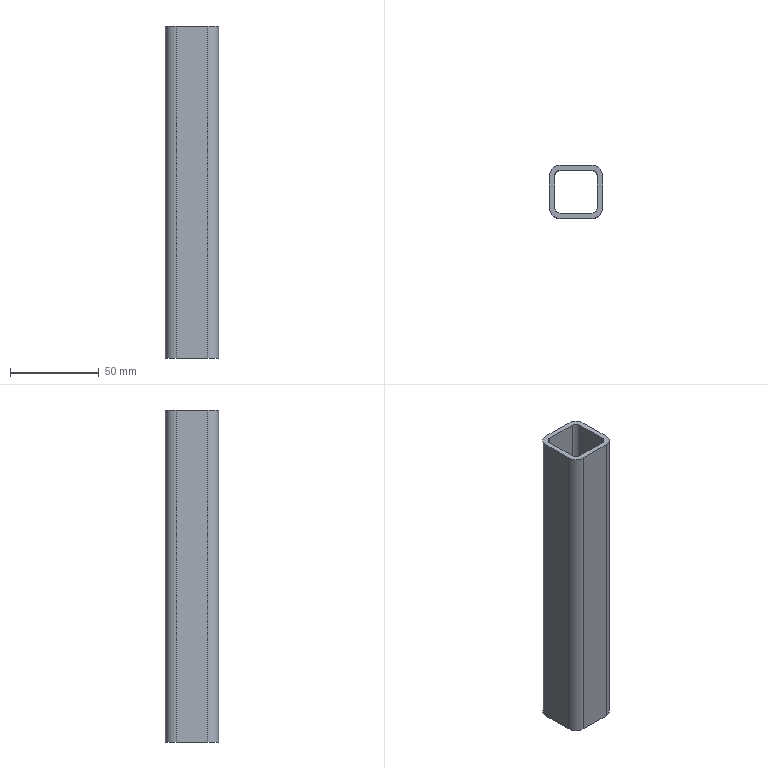Part | SolidWorks | features Attribute 1, Extrusion 1 | 1 solid | 18 faces | box 30 x 30 x 187 mm | volume 56254 mm3 | plane 10 | cylinder 8 | commonest cylinder face diameters 6 x4 12 x4
STEP:
#1=CARTESIAN_POINT('',(-15.,-9.,187.));
#2=VERTEX_POINT('',#1);
#3=CARTESIAN_POINT('',(-9.,-15.,187.));
#4=VERTEX_POINT('',#3);
#5=CARTESIAN_POINT('',(-9.,-9.,187.));
#6=DIRECTION('',(0.,0.,1.));
#7=DIRECTION('',(1.,0.,0.));
#8=AXIS2_PLACEMENT_3D('',#5,#6,#7);
#9=CIRCLE('',#8,6.);
#10=EDGE_CURVE('',#2,#4,#9,.T.);
#11=ORIENTED_EDGE('',*,*,#10,.T.);
#12=CARTESIAN_POINT('',(9.,-15.,187.));
#13=VERTEX_POINT('',#12);
#14=CARTESIAN_POINT('',(-9.,-15.,187.));
#15=DIRECTION('',(1.,0.,0.));
#16=VECTOR('',#15,1000.);
#17=LINE('',#14,#16);
#18=EDGE_CURVE('',#4,#13,#17,.T.);
#19=ORIENTED_EDGE('',*,*,#18,.T.);
#20=CARTESIAN_POINT('',(15.,-9.,187.));
#21=VERTEX_POINT('',#20);
#22=CARTESIAN_POINT('',(9.,-9.,187.));
#23=DIRECTION('',(0.,0.,1.));
#24=DIRECTION('',(1.,0.,0.));
#25=AXIS2_PLACEMENT_3D('',#22,#23,#24);
#26=CIRCLE('',#25,6.);
#27=EDGE_CURVE('',#13,#21,#26,.T.);
#28=ORIENTED_EDGE('',*,*,#27,.T.);
#29=CARTESIAN_POINT('',(15.,9.,187.));
#30=VERTEX_POINT('',#29);
#31=CARTESIAN_POINT('',(15.,9.,187.));
#32=DIRECTION('',(0.,-1.,0.));
#33=VECTOR('',#32,1000.);
#34=LINE('',#31,#33);
#35=EDGE_CURVE('',#30,#21,#34,.T.);
#36=ORIENTED_EDGE('',*,*,#35,.F.);
#37=CARTESIAN_POINT('',(9.,15.,187.));
#38=VERTEX_POINT('',#37);
#39=CARTESIAN_POINT('',(9.,9.,187.));
#40=DIRECTION('',(0.,0.,1.));
#41=DIRECTION('',(1.,0.,0.));
#42=AXIS2_PLACEMENT_3D('',#39,#40,#41);
#43=CIRCLE('',#42,6.);
#44=EDGE_CURVE('',#30,#38,#43,.T.);
#45=ORIENTED_EDGE('',*,*,#44,.T.);
#46=CARTESIAN_POINT('',(-9.,15.,187.));
#47=VERTEX_POINT('',#46);
#48=CARTESIAN_POINT('',(9.,15.,187.));
#49=DIRECTION('',(-1.,0.,0.));
#50=VECTOR('',#49,1000.);
#51=LINE('',#48,#50);
#52=EDGE_CURVE('',#38,#47,#51,.T.);
#53=ORIENTED_EDGE('',*,*,#52,.T.);
#54=CARTESIAN_POINT('',(-15.,9.,187.));
#55=VERTEX_POINT('',#54);
#56=CARTESIAN_POINT('',(-9.,9.,187.));
#57=DIRECTION('',(0.,0.,1.));
#58=DIRECTION('',(1.,0.,0.));
#59=AXIS2_PLACEMENT_3D('',#56,#57,#58);
#60=CIRCLE('',#59,6.);
#61=EDGE_CURVE('',#47,#55,#60,.T.);
#62=ORIENTED_EDGE('',*,*,#61,.T.);
#63=CARTESIAN_POINT('',(-15.,-9.,187.));
#64=DIRECTION('',(0.,1.,0.));
#65=VECTOR('',#64,1000.);
#66=LINE('',#63,#65);
#67=EDGE_CURVE('',#2,#55,#66,.T.);
#68=ORIENTED_EDGE('',*,*,#67,.F.);
#69=EDGE_LOOP('',(#11,#19,#28,#36,#45,#53,#62,#68));
#70=FACE_OUTER_BOUND('',#69,.T.);
#71=CARTESIAN_POINT('',(-9.,-12.,187.));
#72=VERTEX_POINT('',#71);
#73=CARTESIAN_POINT('',(9.,-12.,187.));
#74=VERTEX_POINT('',#73);
#75=CARTESIAN_POINT('',(-9.,-12.,187.));
#76=DIRECTION('',(1.,0.,0.));
#77=VECTOR('',#76,1000.);
#78=LINE('',#75,#77);
#79=EDGE_CURVE('',#72,#74,#78,.T.);
#80=ORIENTED_EDGE('',*,*,#79,.F.);
#81=CARTESIAN_POINT('',(-12.,-9.,187.));
#82=VERTEX_POINT('',#81);
#83=CARTESIAN_POINT('',(-9.,-9.,187.));
#84=DIRECTION('',(0.,0.,1.));
#85=DIRECTION('',(1.,0.,0.));
#86=AXIS2_PLACEMENT_3D('',#83,#84,#85);
#87=CIRCLE('',#86,3.);
#88=EDGE_CURVE('',#82,#72,#87,.T.);
#89=ORIENTED_EDGE('',*,*,#88,.F.);
#90=CARTESIAN_POINT('',(-12.,9.,187.));
#91=VERTEX_POINT('',#90);
#92=CARTESIAN_POINT('',(-12.,-9.,187.));
#93=DIRECTION('',(0.,1.,0.));
#94=VECTOR('',#93,1000.);
#95=LINE('',#92,#94);
#96=EDGE_CURVE('',#82,#91,#95,.T.);
#97=ORIENTED_EDGE('',*,*,#96,.T.);
#98=CARTESIAN_POINT('',(-9.,12.,187.));
#99=VERTEX_POINT('',#98);
#100=CARTESIAN_POINT('',(-9.,9.,187.));
#101=DIRECTION('',(0.,0.,1.));
#102=DIRECTION('',(1.,0.,0.));
#103=AXIS2_PLACEMENT_3D('',#100,#101,#102);
#104=CIRCLE('',#103,3.);
#105=EDGE_CURVE('',#99,#91,#104,.T.);
#106=ORIENTED_EDGE('',*,*,#105,.F.);
#107=CARTESIAN_POINT('',(9.,12.,187.));
#108=VERTEX_POINT('',#107);
#109=CARTESIAN_POINT('',(9.,12.,187.));
#110=DIRECTION('',(-1.,0.,0.));
#111=VECTOR('',#110,1000.);
#112=LINE('',#109,#111);
#113=EDGE_CURVE('',#108,#99,#112,.T.);
#114=ORIENTED_EDGE('',*,*,#113,.F.);
#115=CARTESIAN_POINT('',(12.,9.,187.));
#116=VERTEX_POINT('',#115);
#117=CARTESIAN_POINT('',(9.,9.,187.));
#118=DIRECTION('',(0.,0.,1.));
#119=DIRECTION('',(1.,0.,0.));
#120=AXIS2_PLACEMENT_3D('',#117,#118,#119);
#121=CIRCLE('',#120,3.);
#122=EDGE_CURVE('',#116,#108,#121,.T.);
#123=ORIENTED_EDGE('',*,*,#122,.F.);
#124=CARTESIAN_POINT('',(12.,-9.,187.));
#125=VERTEX_POINT('',#124);
#126=CARTESIAN_POINT('',(12.,9.,187.));
#127=DIRECTION('',(0.,-1.,0.));
#128=VECTOR('',#127,1000.);
#129=LINE('',#126,#128);
#130=EDGE_CURVE('',#116,#125,#129,.T.);
#131=ORIENTED_EDGE('',*,*,#130,.T.);
#132=CARTESIAN_POINT('',(9.,-9.,187.));
#133=DIRECTION('',(0.,0.,1.));
#134=DIRECTION('',(1.,0.,0.));
#135=AXIS2_PLACEMENT_3D('',#132,#133,#134);
#136=CIRCLE('',#135,3.);
#137=EDGE_CURVE('',#74,#125,#136,.T.);
#138=ORIENTED_EDGE('',*,*,#137,.F.);
#139=EDGE_LOOP('',(#80,#89,#97,#106,#114,#123,#131,#138));
#140=FACE_BOUND('',#139,.T.);
#141=CARTESIAN_POINT('',(-9.,-9.,187.));
#142=DIRECTION('',(0.,0.,1.));
#143=DIRECTION('',(1.,0.,0.));
#144=AXIS2_PLACEMENT_3D('',#141,#142,#143);
#145=PLANE('',#144);
#146=ADVANCED_FACE('',(#70,#140),#145,.T.);
#147=CARTESIAN_POINT('',(-15.,-9.,0.));
#148=VERTEX_POINT('',#147);
#149=CARTESIAN_POINT('',(-9.,-15.,0.));
#150=VERTEX_POINT('',#149);
#151=CARTESIAN_POINT('',(-9.,-9.,0.));
#152=DIRECTION('',(0.,0.,1.));
#153=DIRECTION('',(1.,0.,0.));
#154=AXIS2_PLACEMENT_3D('',#151,#152,#153);
#155=CIRCLE('',#154,6.);
#156=EDGE_CURVE('',#148,#150,#155,.T.);
#157=ORIENTED_EDGE('',*,*,#156,.F.);
#158=CARTESIAN_POINT('',(-15.,9.,0.));
#159=VERTEX_POINT('',#158);
#160=CARTESIAN_POINT('',(-15.,-9.,0.));
#161=DIRECTION('',(0.,1.,0.));
#162=VECTOR('',#161,1000.);
#163=LINE('',#160,#162);
#164=EDGE_CURVE('',#148,#159,#163,.T.);
#165=ORIENTED_EDGE('',*,*,#164,.T.);
#166=CARTESIAN_POINT('',(-9.,15.,0.));
#167=VERTEX_POINT('',#166);
#168=CARTESIAN_POINT('',(-9.,9.,0.));
#169=DIRECTION('',(0.,0.,1.));
#170=DIRECTION('',(1.,0.,0.));
#171=AXIS2_PLACEMENT_3D('',#168,#169,#170);
#172=CIRCLE('',#171,6.);
#173=EDGE_CURVE('',#167,#159,#172,.T.);
#174=ORIENTED_EDGE('',*,*,#173,.F.);
#175=CARTESIAN_POINT('',(9.,15.,0.));
#176=VERTEX_POINT('',#175);
#177=CARTESIAN_POINT('',(9.,15.,0.));
#178=DIRECTION('',(-1.,0.,0.));
#179=VECTOR('',#178,1000.);
#180=LINE('',#177,#179);
#181=EDGE_CURVE('',#176,#167,#180,.T.);
#182=ORIENTED_EDGE('',*,*,#181,.F.);
#183=CARTESIAN_POINT('',(15.,9.,0.));
#184=VERTEX_POINT('',#183);
#185=CARTESIAN_POINT('',(9.,9.,0.));
#186=DIRECTION('',(0.,0.,1.));
#187=DIRECTION('',(1.,0.,0.));
#188=AXIS2_PLACEMENT_3D('',#185,#186,#187);
#189=CIRCLE('',#188,6.);
#190=EDGE_CURVE('',#184,#176,#189,.T.);
#191=ORIENTED_EDGE('',*,*,#190,.F.);
#192=CARTESIAN_POINT('',(15.,-9.,0.));
#193=VERTEX_POINT('',#192);
#194=CARTESIAN_POINT('',(15.,9.,0.));
#195=DIRECTION('',(0.,-1.,0.));
#196=VECTOR('',#195,1000.);
#197=LINE('',#194,#196);
#198=EDGE_CURVE('',#184,#193,#197,.T.);
#199=ORIENTED_EDGE('',*,*,#198,.T.);
#200=CARTESIAN_POINT('',(9.,-15.,0.));
#201=VERTEX_POINT('',#200);
#202=CARTESIAN_POINT('',(9.,-9.,0.));
#203=DIRECTION('',(0.,0.,1.));
#204=DIRECTION('',(1.,0.,0.));
#205=AXIS2_PLACEMENT_3D('',#202,#203,#204);
#206=CIRCLE('',#205,6.);
#207=EDGE_CURVE('',#201,#193,#206,.T.);
#208=ORIENTED_EDGE('',*,*,#207,.F.);
#209=CARTESIAN_POINT('',(-9.,-15.,0.));
#210=DIRECTION('',(1.,0.,0.));
#211=VECTOR('',#210,1000.);
#212=LINE('',#209,#211);
#213=EDGE_CURVE('',#150,#201,#212,.T.);
#214=ORIENTED_EDGE('',*,*,#213,.F.);
#215=EDGE_LOOP('',(#157,#165,#174,#182,#191,#199,#208,#214));
#216=FACE_OUTER_BOUND('',#215,.T.);
#217=CARTESIAN_POINT('',(-12.,-9.,0.));
#218=VERTEX_POINT('',#217);
#219=CARTESIAN_POINT('',(-9.,-12.,0.));
#220=VERTEX_POINT('',#219);
#221=CARTESIAN_POINT('',(-9.,-9.,0.));
#222=DIRECTION('',(0.,0.,1.));
#223=DIRECTION('',(1.,0.,0.));
#224=AXIS2_PLACEMENT_3D('',#221,#222,#223);
#225=CIRCLE('',#224,3.);
#226=EDGE_CURVE('',#218,#220,#225,.T.);
#227=ORIENTED_EDGE('',*,*,#226,.T.);
#228=CARTESIAN_POINT('',(9.,-12.,0.));
#229=VERTEX_POINT('',#228);
#230=CARTESIAN_POINT('',(-9.,-12.,0.));
#231=DIRECTION('',(1.,0.,0.));
#232=VECTOR('',#231,1000.);
#233=LINE('',#230,#232);
#234=EDGE_CURVE('',#220,#229,#233,.T.);
#235=ORIENTED_EDGE('',*,*,#234,.T.);
#236=CARTESIAN_POINT('',(12.,-9.,0.));
#237=VERTEX_POINT('',#236);
#238=CARTESIAN_POINT('',(9.,-9.,0.));
#239=DIRECTION('',(0.,0.,1.));
#240=DIRECTION('',(1.,0.,0.));
#241=AXIS2_PLACEMENT_3D('',#238,#239,#240);
#242=CIRCLE('',#241,3.);
#243=EDGE_CURVE('',#229,#237,#242,.T.);
#244=ORIENTED_EDGE('',*,*,#243,.T.);
#245=CARTESIAN_POINT('',(12.,9.,0.));
#246=VERTEX_POINT('',#245);
#247=CARTESIAN_POINT('',(12.,9.,0.));
#248=DIRECTION('',(0.,-1.,0.));
#249=VECTOR('',#248,1000.);
#250=LINE('',#247,#249);
#251=EDGE_CURVE('',#246,#237,#250,.T.);
#252=ORIENTED_EDGE('',*,*,#251,.F.);
#253=CARTESIAN_POINT('',(9.,12.,0.));
#254=VERTEX_POINT('',#253);
#255=CARTESIAN_POINT('',(9.,9.,0.));
#256=DIRECTION('',(0.,0.,1.));
#257=DIRECTION('',(1.,0.,0.));
#258=AXIS2_PLACEMENT_3D('',#255,#256,#257);
#259=CIRCLE('',#258,3.);
#260=EDGE_CURVE('',#246,#254,#259,.T.);
#261=ORIENTED_EDGE('',*,*,#260,.T.);
#262=CARTESIAN_POINT('',(-9.,12.,0.));
#263=VERTEX_POINT('',#262);
#264=CARTESIAN_POINT('',(9.,12.,0.));
#265=DIRECTION('',(-1.,0.,0.));
#266=VECTOR('',#265,1000.);
#267=LINE('',#264,#266);
#268=EDGE_CURVE('',#254,#263,#267,.T.);
#269=ORIENTED_EDGE('',*,*,#268,.T.);
#270=CARTESIAN_POINT('',(-12.,9.,0.));
#271=VERTEX_POINT('',#270);
#272=CARTESIAN_POINT('',(-9.,9.,0.));
#273=DIRECTION('',(0.,0.,1.));
#274=DIRECTION('',(1.,0.,0.));
#275=AXIS2_PLACEMENT_3D('',#272,#273,#274);
#276=CIRCLE('',#275,3.);
#277=EDGE_CURVE('',#263,#271,#276,.T.);
#278=ORIENTED_EDGE('',*,*,#277,.T.);
#279=CARTESIAN_POINT('',(-12.,-9.,0.));
#280=DIRECTION('',(0.,1.,0.));
#281=VECTOR('',#280,1000.);
#282=LINE('',#279,#281);
#283=EDGE_CURVE('',#218,#271,#282,.T.);
#284=ORIENTED_EDGE('',*,*,#283,.F.);
#285=EDGE_LOOP('',(#227,#235,#244,#252,#261,#269,#278,#284));
#286=FACE_BOUND('',#285,.T.);
#287=CARTESIAN_POINT('',(-9.,-9.,0.));
#288=DIRECTION('',(0.,0.,1.));
#289=DIRECTION('',(1.,0.,0.));
#290=AXIS2_PLACEMENT_3D('',#287,#288,#289);
#291=PLANE('',#290);
#292=ADVANCED_FACE('',(#216,#286),#291,.F.);
#293=ORIENTED_EDGE('',*,*,#156,.T.);
#294=CARTESIAN_POINT('',(-9.,-15.,187.));
#295=DIRECTION('',(0.,0.,-1.));
#296=VECTOR('',#295,1000.);
#297=LINE('',#294,#296);
#298=EDGE_CURVE('',#4,#150,#297,.T.);
#299=ORIENTED_EDGE('',*,*,#298,.F.);
#300=ORIENTED_EDGE('',*,*,#10,.F.);
#301=CARTESIAN_POINT('',(-15.,-9.,187.));
#302=DIRECTION('',(0.,0.,-1.));
#303=VECTOR('',#302,1000.);
#304=LINE('',#301,#303);
#305=EDGE_CURVE('',#2,#148,#304,.T.);
#306=ORIENTED_EDGE('',*,*,#305,.T.);
#307=EDGE_LOOP('',(#293,#299,#300,#306));
#308=FACE_OUTER_BOUND('',#307,.T.);
#309=CARTESIAN_POINT('',(-9.,-9.,187.));
#310=DIRECTION('',(0.,0.,-1.));
#311=DIRECTION('',(-1.,0.,0.));
#312=AXIS2_PLACEMENT_3D('',#309,#310,#311);
#313=CYLINDRICAL_SURFACE('',#312,6.);
#314=ADVANCED_FACE('',(#308),#313,.T.);
#315=ORIENTED_EDGE('',*,*,#213,.T.);
#316=CARTESIAN_POINT('',(9.,-15.,187.));
#317=DIRECTION('',(0.,0.,-1.));
#318=VECTOR('',#317,1000.);
#319=LINE('',#316,#318);
#320=EDGE_CURVE('',#13,#201,#319,.T.);
#321=ORIENTED_EDGE('',*,*,#320,.F.);
#322=ORIENTED_EDGE('',*,*,#18,.F.);
#323=ORIENTED_EDGE('',*,*,#298,.T.);
#324=EDGE_LOOP('',(#315,#321,#322,#323));
#325=FACE_OUTER_BOUND('',#324,.T.);
#326=CARTESIAN_POINT('',(-9.,-15.,187.));
#327=DIRECTION('',(0.,1.,0.));
#328=DIRECTION('',(0.,0.,1.));
#329=AXIS2_PLACEMENT_3D('',#326,#327,#328);
#330=PLANE('',#329);
#331=ADVANCED_FACE('',(#325),#330,.F.);
#332=ORIENTED_EDGE('',*,*,#207,.T.);
#333=CARTESIAN_POINT('',(15.,-9.,187.));
#334=DIRECTION('',(0.,0.,-1.));
#335=VECTOR('',#334,1000.);
#336=LINE('',#333,#335);
#337=EDGE_CURVE('',#21,#193,#336,.T.);
#338=ORIENTED_EDGE('',*,*,#337,.F.);
#339=ORIENTED_EDGE('',*,*,#27,.F.);
#340=ORIENTED_EDGE('',*,*,#320,.T.);
#341=EDGE_LOOP('',(#332,#338,#339,#340));
#342=FACE_OUTER_BOUND('',#341,.T.);
#343=CARTESIAN_POINT('',(9.,-9.,187.));
#344=DIRECTION('',(0.,0.,-1.));
#345=DIRECTION('',(-1.,0.,0.));
#346=AXIS2_PLACEMENT_3D('',#343,#344,#345);
#347=CYLINDRICAL_SURFACE('',#346,6.);
#348=ADVANCED_FACE('',(#342),#347,.T.);
#349=ORIENTED_EDGE('',*,*,#198,.F.);
#350=CARTESIAN_POINT('',(15.,9.,187.));
#351=DIRECTION('',(0.,0.,-1.));
#352=VECTOR('',#351,1000.);
#353=LINE('',#350,#352);
#354=EDGE_CURVE('',#30,#184,#353,.T.);
#355=ORIENTED_EDGE('',*,*,#354,.F.);
#356=ORIENTED_EDGE('',*,*,#35,.T.);
#357=ORIENTED_EDGE('',*,*,#337,.T.);
#358=EDGE_LOOP('',(#349,#355,#356,#357));
#359=FACE_OUTER_BOUND('',#358,.T.);
#360=CARTESIAN_POINT('',(15.,9.,187.));
#361=DIRECTION('',(1.,0.,0.));
#362=DIRECTION('',(0.,0.,-1.));
#363=AXIS2_PLACEMENT_3D('',#360,#361,#362);
#364=PLANE('',#363);
#365=ADVANCED_FACE('',(#359),#364,.T.);
#366=ORIENTED_EDGE('',*,*,#190,.T.);
#367=CARTESIAN_POINT('',(9.,15.,187.));
#368=DIRECTION('',(0.,0.,-1.));
#369=VECTOR('',#368,1000.);
#370=LINE('',#367,#369);
#371=EDGE_CURVE('',#38,#176,#370,.T.);
#372=ORIENTED_EDGE('',*,*,#371,.F.);
#373=ORIENTED_EDGE('',*,*,#44,.F.);
#374=ORIENTED_EDGE('',*,*,#354,.T.);
#375=EDGE_LOOP('',(#366,#372,#373,#374));
#376=FACE_OUTER_BOUND('',#375,.T.);
#377=CARTESIAN_POINT('',(9.,9.,187.));
#378=DIRECTION('',(0.,0.,-1.));
#379=DIRECTION('',(-1.,0.,0.));
#380=AXIS2_PLACEMENT_3D('',#377,#378,#379);
#381=CYLINDRICAL_SURFACE('',#380,6.);
#382=ADVANCED_FACE('',(#376),#381,.T.);
#383=ORIENTED_EDGE('',*,*,#181,.T.);
#384=CARTESIAN_POINT('',(-9.,15.,187.));
#385=DIRECTION('',(0.,0.,-1.));
#386=VECTOR('',#385,1000.);
#387=LINE('',#384,#386);
#388=EDGE_CURVE('',#47,#167,#387,.T.);
#389=ORIENTED_EDGE('',*,*,#388,.F.);
#390=ORIENTED_EDGE('',*,*,#52,.F.);
#391=ORIENTED_EDGE('',*,*,#371,.T.);
#392=EDGE_LOOP('',(#383,#389,#390,#391));
#393=FACE_OUTER_BOUND('',#392,.T.);
#394=CARTESIAN_POINT('',(9.,15.,187.));
#395=DIRECTION('',(0.,-1.,0.));
#396=DIRECTION('',(0.,0.,-1.));
#397=AXIS2_PLACEMENT_3D('',#394,#395,#396);
#398=PLANE('',#397);
#399=ADVANCED_FACE('',(#393),#398,.F.);
#400=ORIENTED_EDGE('',*,*,#173,.T.);
#401=CARTESIAN_POINT('',(-15.,9.,187.));
#402=DIRECTION('',(0.,0.,-1.));
#403=VECTOR('',#402,1000.);
#404=LINE('',#401,#403);
#405=EDGE_CURVE('',#55,#159,#404,.T.);
#406=ORIENTED_EDGE('',*,*,#405,.F.);
#407=ORIENTED_EDGE('',*,*,#61,.F.);
#408=ORIENTED_EDGE('',*,*,#388,.T.);
#409=EDGE_LOOP('',(#400,#406,#407,#408));
#410=FACE_OUTER_BOUND('',#409,.T.);
#411=CARTESIAN_POINT('',(-9.,9.,187.));
#412=DIRECTION('',(0.,0.,-1.));
#413=DIRECTION('',(-1.,0.,0.));
#414=AXIS2_PLACEMENT_3D('',#411,#412,#413);
#415=CYLINDRICAL_SURFACE('',#414,6.);
#416=ADVANCED_FACE('',(#410),#415,.T.);
#417=ORIENTED_EDGE('',*,*,#164,.F.);
#418=ORIENTED_EDGE('',*,*,#305,.F.);
#419=ORIENTED_EDGE('',*,*,#67,.T.);
#420=ORIENTED_EDGE('',*,*,#405,.T.);
#421=EDGE_LOOP('',(#417,#418,#419,#420));
#422=FACE_OUTER_BOUND('',#421,.T.);
#423=CARTESIAN_POINT('',(-15.,-9.,187.));
#424=DIRECTION('',(-1.,0.,0.));
#425=DIRECTION('',(0.,0.,1.));
#426=AXIS2_PLACEMENT_3D('',#423,#424,#425);
#427=PLANE('',#426);
#428=ADVANCED_FACE('',(#422),#427,.T.);
#429=ORIENTED_EDGE('',*,*,#226,.F.);
#430=CARTESIAN_POINT('',(-12.,-9.,187.));
#431=DIRECTION('',(0.,0.,-1.));
#432=VECTOR('',#431,1000.);
#433=LINE('',#430,#432);
#434=EDGE_CURVE('',#82,#218,#433,.T.);
#435=ORIENTED_EDGE('',*,*,#434,.F.);
#436=ORIENTED_EDGE('',*,*,#88,.T.);
#437=CARTESIAN_POINT('',(-9.,-12.,187.));
#438=DIRECTION('',(0.,0.,-1.));
#439=VECTOR('',#438,1000.);
#440=LINE('',#437,#439);
#441=EDGE_CURVE('',#72,#220,#440,.T.);
#442=ORIENTED_EDGE('',*,*,#441,.T.);
#443=EDGE_LOOP('',(#429,#435,#436,#442));
#444=FACE_OUTER_BOUND('',#443,.T.);
#445=CARTESIAN_POINT('',(-9.,-9.,187.));
#446=DIRECTION('',(0.,0.,-1.));
#447=DIRECTION('',(-1.,0.,0.));
#448=AXIS2_PLACEMENT_3D('',#445,#446,#447);
#449=CYLINDRICAL_SURFACE('',#448,3.);
#450=ADVANCED_FACE('',(#444),#449,.F.);
#451=ORIENTED_EDGE('',*,*,#234,.F.);
#452=ORIENTED_EDGE('',*,*,#441,.F.);
#453=ORIENTED_EDGE('',*,*,#79,.T.);
#454=CARTESIAN_POINT('',(9.,-12.,187.));
#455=DIRECTION('',(0.,0.,-1.));
#456=VECTOR('',#455,1000.);
#457=LINE('',#454,#456);
#458=EDGE_CURVE('',#74,#229,#457,.T.);
#459=ORIENTED_EDGE('',*,*,#458,.T.);
#460=EDGE_LOOP('',(#451,#452,#453,#459));
#461=FACE_OUTER_BOUND('',#460,.T.);
#462=CARTESIAN_POINT('',(-9.,-12.,187.));
#463=DIRECTION('',(0.,1.,0.));
#464=DIRECTION('',(0.,0.,1.));
#465=AXIS2_PLACEMENT_3D('',#462,#463,#464);
#466=PLANE('',#465);
#467=ADVANCED_FACE('',(#461),#466,.T.);
#468=ORIENTED_EDGE('',*,*,#243,.F.);
#469=ORIENTED_EDGE('',*,*,#458,.F.);
#470=ORIENTED_EDGE('',*,*,#137,.T.);
#471=CARTESIAN_POINT('',(12.,-9.,187.));
#472=DIRECTION('',(0.,0.,-1.));
#473=VECTOR('',#472,1000.);
#474=LINE('',#471,#473);
#475=EDGE_CURVE('',#125,#237,#474,.T.);
#476=ORIENTED_EDGE('',*,*,#475,.T.);
#477=EDGE_LOOP('',(#468,#469,#470,#476));
#478=FACE_OUTER_BOUND('',#477,.T.);
#479=CARTESIAN_POINT('',(9.,-9.,187.));
#480=DIRECTION('',(0.,0.,-1.));
#481=DIRECTION('',(-1.,0.,0.));
#482=AXIS2_PLACEMENT_3D('',#479,#480,#481);
#483=CYLINDRICAL_SURFACE('',#482,3.);
#484=ADVANCED_FACE('',(#478),#483,.F.);
#485=ORIENTED_EDGE('',*,*,#251,.T.);
#486=ORIENTED_EDGE('',*,*,#475,.F.);
#487=ORIENTED_EDGE('',*,*,#130,.F.);
#488=CARTESIAN_POINT('',(12.,9.,187.));
#489=DIRECTION('',(0.,0.,-1.));
#490=VECTOR('',#489,1000.);
#491=LINE('',#488,#490);
#492=EDGE_CURVE('',#116,#246,#491,.T.);
#493=ORIENTED_EDGE('',*,*,#492,.T.);
#494=EDGE_LOOP('',(#485,#486,#487,#493));
#495=FACE_OUTER_BOUND('',#494,.T.);
#496=CARTESIAN_POINT('',(12.,9.,187.));
#497=DIRECTION('',(1.,0.,0.));
#498=DIRECTION('',(0.,0.,-1.));
#499=AXIS2_PLACEMENT_3D('',#496,#497,#498);
#500=PLANE('',#499);
#501=ADVANCED_FACE('',(#495),#500,.F.);
#502=ORIENTED_EDGE('',*,*,#260,.F.);
#503=ORIENTED_EDGE('',*,*,#492,.F.);
#504=ORIENTED_EDGE('',*,*,#122,.T.);
#505=CARTESIAN_POINT('',(9.,12.,187.));
#506=DIRECTION('',(0.,0.,-1.));
#507=VECTOR('',#506,1000.);
#508=LINE('',#505,#507);
#509=EDGE_CURVE('',#108,#254,#508,.T.);
#510=ORIENTED_EDGE('',*,*,#509,.T.);
#511=EDGE_LOOP('',(#502,#503,#504,#510));
#512=FACE_OUTER_BOUND('',#511,.T.);
#513=CARTESIAN_POINT('',(9.,9.,187.));
#514=DIRECTION('',(0.,0.,-1.));
#515=DIRECTION('',(-1.,0.,0.));
#516=AXIS2_PLACEMENT_3D('',#513,#514,#515);
#517=CYLINDRICAL_SURFACE('',#516,3.);
#518=ADVANCED_FACE('',(#512),#517,.F.);
#519=ORIENTED_EDGE('',*,*,#268,.F.);
#520=ORIENTED_EDGE('',*,*,#509,.F.);
#521=ORIENTED_EDGE('',*,*,#113,.T.);
#522=CARTESIAN_POINT('',(-9.,12.,187.));
#523=DIRECTION('',(0.,0.,-1.));
#524=VECTOR('',#523,1000.);
#525=LINE('',#522,#524);
#526=EDGE_CURVE('',#99,#263,#525,.T.);
#527=ORIENTED_EDGE('',*,*,#526,.T.);
#528=EDGE_LOOP('',(#519,#520,#521,#527));
#529=FACE_OUTER_BOUND('',#528,.T.);
#530=CARTESIAN_POINT('',(9.,12.,187.));
#531=DIRECTION('',(0.,-1.,0.));
#532=DIRECTION('',(0.,0.,-1.));
#533=AXIS2_PLACEMENT_3D('',#530,#531,#532);
#534=PLANE('',#533);
#535=ADVANCED_FACE('',(#529),#534,.T.);
#536=ORIENTED_EDGE('',*,*,#277,.F.);
#537=ORIENTED_EDGE('',*,*,#526,.F.);
#538=ORIENTED_EDGE('',*,*,#105,.T.);
#539=CARTESIAN_POINT('',(-12.,9.,187.));
#540=DIRECTION('',(0.,0.,-1.));
#541=VECTOR('',#540,1000.);
#542=LINE('',#539,#541);
#543=EDGE_CURVE('',#91,#271,#542,.T.);
#544=ORIENTED_EDGE('',*,*,#543,.T.);
#545=EDGE_LOOP('',(#536,#537,#538,#544));
#546=FACE_OUTER_BOUND('',#545,.T.);
#547=CARTESIAN_POINT('',(-9.,9.,187.));
#548=DIRECTION('',(0.,0.,-1.));
#549=DIRECTION('',(-1.,0.,0.));
#550=AXIS2_PLACEMENT_3D('',#547,#548,#549);
#551=CYLINDRICAL_SURFACE('',#550,3.);
#552=ADVANCED_FACE('',(#546),#551,.F.);
#553=ORIENTED_EDGE('',*,*,#283,.T.);
#554=ORIENTED_EDGE('',*,*,#543,.F.);
#555=ORIENTED_EDGE('',*,*,#96,.F.);
#556=ORIENTED_EDGE('',*,*,#434,.T.);
#557=EDGE_LOOP('',(#553,#554,#555,#556));
#558=FACE_OUTER_BOUND('',#557,.T.);
#559=CARTESIAN_POINT('',(-12.,-9.,187.));
#560=DIRECTION('',(-1.,0.,0.));
#561=DIRECTION('',(0.,0.,1.));
#562=AXIS2_PLACEMENT_3D('',#559,#560,#561);
#563=PLANE('',#562);
#564=ADVANCED_FACE('',(#558),#563,.F.);
#565=CLOSED_SHELL('',(#146,#292,#314,#331,#348,#365,#382,#399,#416,#428,#450,#467,#484,#501,#518,#535,#552,#564));
#566=MANIFOLD_SOLID_BREP('',#565);
#567=CARTESIAN_POINT('',(0.,0.,0.));
#568=DIRECTION('',(0.,0.,1.));
#569=DIRECTION('',(1.,0.,0.));
#570=AXIS2_PLACEMENT_3D('',#567,#568,#569);
#571=(LENGTH_UNIT()NAMED_UNIT(*)SI_UNIT(.MILLI.,.METRE.));
#572=UNCERTAINTY_MEASURE_WITH_UNIT(LENGTH_MEASURE(0.00001),#571,'','');
#573=(NAMED_UNIT(*)PLANE_ANGLE_UNIT()SI_UNIT($,.RADIAN.));
#574=(NAMED_UNIT(*)SI_UNIT($,.STERADIAN.)SOLID_ANGLE_UNIT());
#575=(GEOMETRIC_REPRESENTATION_CONTEXT(3)GLOBAL_UNCERTAINTY_ASSIGNED_CONTEXT((#572))GLOBAL_UNIT_ASSIGNED_CONTEXT((#571,#573,#574))REPRESENTATION_CONTEXT('',''));
#576=ADVANCED_BREP_SHAPE_REPRESENTATION('',(#566,#570),#575);